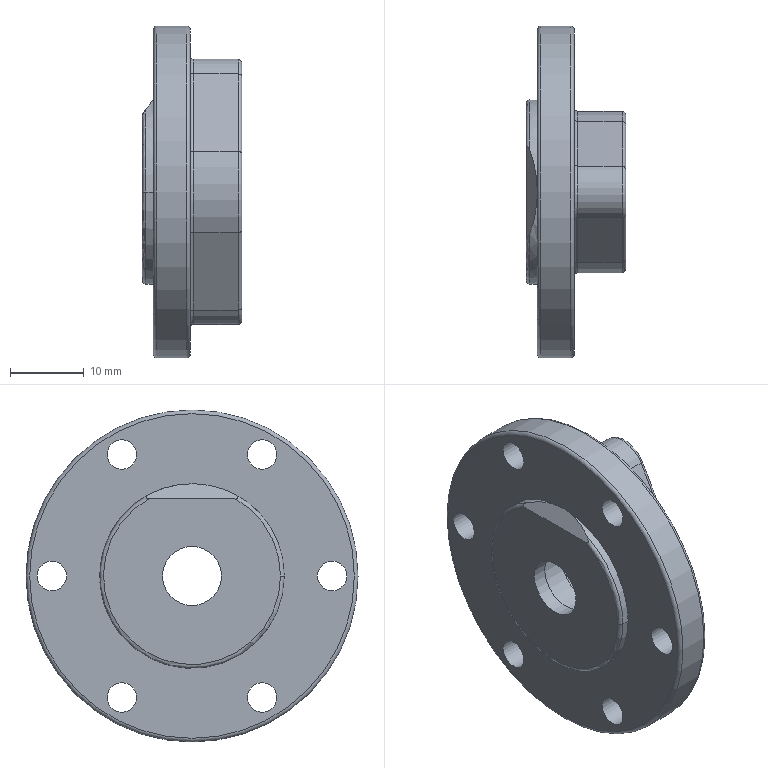Part | STEP file | 1-08.1 | 1 solid | 51 faces | box 13.5 x 45 x 45 mm | volume 10498 mm3 | cylinder 26 | plane 13 | torus 12 | commonest cylinder face diameters 1 x8 4 x8 8 x3 22 x2 25 x2 10 x1